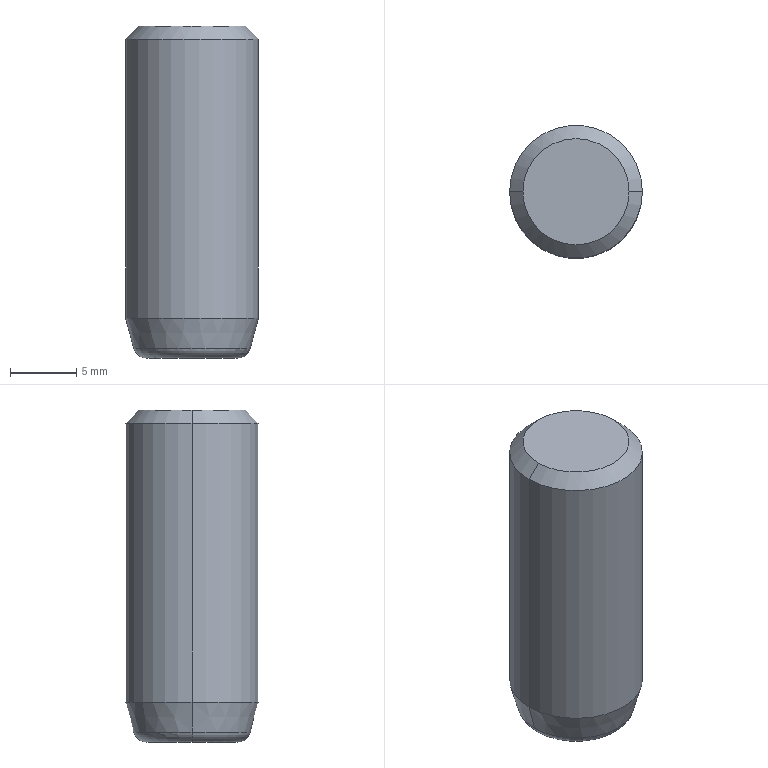Part | NX | features BREP 1 | 1 solid | 10 faces | box 10 x 10 x 25 mm | volume 1910 mm3 | cone 4 | torus 2 | cylinder 2 | plane 2 | commonest cylinder face diameters 10 x2
STEP:
#1=CARTESIAN_POINT('',(-3.429,0.,0.));
#2=VERTEX_POINT('',#1);
#3=CARTESIAN_POINT('',(3.429,0.,0.));
#4=VERTEX_POINT('',#3);
#5=CARTESIAN_POINT('',(0.,0.,0.));
#6=DIRECTION('',(0.,0.,-1.));
#7=DIRECTION('',(1.,0.,0.));
#8=AXIS2_PLACEMENT_3D('',#5,#6,#7);
#9=CIRCLE('',#8,3.429);
#10=EDGE_CURVE('',#2,#4,#9,.T.);
#11=ORIENTED_EDGE('',*,*,#10,.F.);
#12=CARTESIAN_POINT('',(-4.395,0.,0.7412));
#13=VERTEX_POINT('',#12);
#14=CARTESIAN_POINT('',(-3.429,0.,1.));
#15=DIRECTION('',(0.,1.,0.));
#16=DIRECTION('',(-1.,0.,0.));
#17=AXIS2_PLACEMENT_3D('',#14,#15,#16);
#18=CIRCLE('',#17,1.);
#19=EDGE_CURVE('',#13,#2,#18,.F.);
#20=ORIENTED_EDGE('',*,*,#19,.F.);
#21=CARTESIAN_POINT('',(4.395,0.,0.7412));
#22=VERTEX_POINT('',#21);
#23=CARTESIAN_POINT('',(0.,0.,0.7412));
#24=DIRECTION('',(0.,0.,1.));
#25=DIRECTION('',(1.,0.,0.));
#26=AXIS2_PLACEMENT_3D('',#23,#24,#25);
#27=CIRCLE('',#26,4.395);
#28=EDGE_CURVE('',#22,#13,#27,.T.);
#29=ORIENTED_EDGE('',*,*,#28,.F.);
#30=CARTESIAN_POINT('',(3.429,0.,1.));
#31=DIRECTION('',(0.,-1.,0.));
#32=DIRECTION('',(0.,0.,-1.));
#33=AXIS2_PLACEMENT_3D('',#30,#31,#32);
#34=CIRCLE('',#33,1.);
#35=EDGE_CURVE('',#22,#4,#34,.F.);
#36=ORIENTED_EDGE('',*,*,#35,.T.);
#37=EDGE_LOOP('',(#11,#20,#29,#36));
#38=FACE_BOUND('',#37,.T.);
#39=CARTESIAN_POINT('',(0.,0.,1.));
#40=DIRECTION('',(0.,0.,1.));
#41=DIRECTION('',(1.,0.,0.));
#42=AXIS2_PLACEMENT_3D('',#39,#40,#41);
#43=TOROIDAL_SURFACE('',#42,3.429,1.);
#44=ADVANCED_FACE('',(#38),#43,.T.);
#45=ORIENTED_EDGE('',*,*,#28,.T.);
#46=CARTESIAN_POINT('',(-5.,0.,3.));
#47=VERTEX_POINT('',#46);
#48=CARTESIAN_POINT('',(-5.,0.,3.));
#49=DIRECTION('',(-0.2588,0.,0.9659));
#50=VECTOR('',#49,1000.);
#51=LINE('',#48,#50);
#52=EDGE_CURVE('',#47,#13,#51,.F.);
#53=ORIENTED_EDGE('',*,*,#52,.F.);
#54=CARTESIAN_POINT('',(5.,0.,3.));
#55=VERTEX_POINT('',#54);
#56=CARTESIAN_POINT('',(0.,0.,3.));
#57=DIRECTION('',(0.,0.,1.));
#58=DIRECTION('',(1.,0.,0.));
#59=AXIS2_PLACEMENT_3D('',#56,#57,#58);
#60=CIRCLE('',#59,5.);
#61=EDGE_CURVE('',#55,#47,#60,.T.);
#62=ORIENTED_EDGE('',*,*,#61,.F.);
#63=CARTESIAN_POINT('',(5.,0.,3.));
#64=DIRECTION('',(0.2588,0.,0.9659));
#65=VECTOR('',#64,1000.);
#66=LINE('',#63,#65);
#67=EDGE_CURVE('',#55,#22,#66,.F.);
#68=ORIENTED_EDGE('',*,*,#67,.T.);
#69=EDGE_LOOP('',(#45,#53,#62,#68));
#70=FACE_BOUND('',#69,.T.);
#71=CARTESIAN_POINT('',(0.,0.,3.));
#72=DIRECTION('',(0.,0.,1.));
#73=DIRECTION('',(1.,0.,0.));
#74=AXIS2_PLACEMENT_3D('',#71,#72,#73);
#75=CONICAL_SURFACE('',#74,5.,0.2618);
#76=ADVANCED_FACE('',(#70),#75,.T.);
#77=CARTESIAN_POINT('',(4.,0.,25.));
#78=VERTEX_POINT('',#77);
#79=CARTESIAN_POINT('',(-4.,0.,25.));
#80=VERTEX_POINT('',#79);
#81=CARTESIAN_POINT('',(0.,0.,25.));
#82=DIRECTION('',(0.,0.,1.));
#83=DIRECTION('',(1.,0.,0.));
#84=AXIS2_PLACEMENT_3D('',#81,#82,#83);
#85=CIRCLE('',#84,4.);
#86=EDGE_CURVE('',#78,#80,#85,.T.);
#87=ORIENTED_EDGE('',*,*,#86,.F.);
#88=CARTESIAN_POINT('',(5.,0.,24.));
#89=VERTEX_POINT('',#88);
#90=CARTESIAN_POINT('',(4.,0.,25.));
#91=DIRECTION('',(0.7071,0.,-0.7071));
#92=VECTOR('',#91,1000.);
#93=LINE('',#90,#92);
#94=EDGE_CURVE('',#78,#89,#93,.T.);
#95=ORIENTED_EDGE('',*,*,#94,.T.);
#96=CARTESIAN_POINT('',(-5.,0.,24.));
#97=VERTEX_POINT('',#96);
#98=CARTESIAN_POINT('',(0.,0.,24.));
#99=DIRECTION('',(0.,0.,-1.));
#100=DIRECTION('',(1.,0.,0.));
#101=AXIS2_PLACEMENT_3D('',#98,#99,#100);
#102=CIRCLE('',#101,5.);
#103=EDGE_CURVE('',#97,#89,#102,.T.);
#104=ORIENTED_EDGE('',*,*,#103,.F.);
#105=CARTESIAN_POINT('',(-4.,0.,25.));
#106=DIRECTION('',(-0.7071,0.,-0.7071));
#107=VECTOR('',#106,1000.);
#108=LINE('',#105,#107);
#109=EDGE_CURVE('',#80,#97,#108,.T.);
#110=ORIENTED_EDGE('',*,*,#109,.F.);
#111=EDGE_LOOP('',(#87,#95,#104,#110));
#112=FACE_BOUND('',#111,.T.);
#113=CARTESIAN_POINT('',(0.,0.,25.));
#114=DIRECTION('',(0.,0.,-1.));
#115=DIRECTION('',(-1.,0.,0.));
#116=AXIS2_PLACEMENT_3D('',#113,#114,#115);
#117=CONICAL_SURFACE('',#116,4.,0.7854);
#118=ADVANCED_FACE('',(#112),#117,.T.);
#119=ORIENTED_EDGE('',*,*,#103,.T.);
#120=CARTESIAN_POINT('',(5.,0.,25.));
#121=DIRECTION('',(0.,0.,-1.));
#122=VECTOR('',#121,1000.);
#123=LINE('',#120,#122);
#124=EDGE_CURVE('',#89,#55,#123,.T.);
#125=ORIENTED_EDGE('',*,*,#124,.T.);
#126=ORIENTED_EDGE('',*,*,#61,.T.);
#127=CARTESIAN_POINT('',(-5.,0.,25.));
#128=DIRECTION('',(0.,0.,-1.));
#129=VECTOR('',#128,1000.);
#130=LINE('',#127,#129);
#131=EDGE_CURVE('',#97,#47,#130,.T.);
#132=ORIENTED_EDGE('',*,*,#131,.F.);
#133=EDGE_LOOP('',(#119,#125,#126,#132));
#134=FACE_BOUND('',#133,.T.);
#135=CARTESIAN_POINT('',(0.,0.,25.));
#136=DIRECTION('',(0.,0.,-1.));
#137=DIRECTION('',(-1.,0.,0.));
#138=AXIS2_PLACEMENT_3D('',#135,#136,#137);
#139=CYLINDRICAL_SURFACE('',#138,5.);
#140=ADVANCED_FACE('',(#134),#139,.T.);
#141=ORIENTED_EDGE('',*,*,#124,.F.);
#142=CARTESIAN_POINT('',(0.,0.,24.));
#143=DIRECTION('',(0.,0.,-1.));
#144=DIRECTION('',(1.,0.,0.));
#145=AXIS2_PLACEMENT_3D('',#142,#143,#144);
#146=CIRCLE('',#145,5.);
#147=EDGE_CURVE('',#89,#97,#146,.T.);
#148=ORIENTED_EDGE('',*,*,#147,.T.);
#149=ORIENTED_EDGE('',*,*,#131,.T.);
#150=CARTESIAN_POINT('',(0.,0.,3.));
#151=DIRECTION('',(0.,0.,1.));
#152=DIRECTION('',(1.,0.,0.));
#153=AXIS2_PLACEMENT_3D('',#150,#151,#152);
#154=CIRCLE('',#153,5.);
#155=EDGE_CURVE('',#47,#55,#154,.T.);
#156=ORIENTED_EDGE('',*,*,#155,.T.);
#157=EDGE_LOOP('',(#141,#148,#149,#156));
#158=FACE_BOUND('',#157,.T.);
#159=CARTESIAN_POINT('',(0.,0.,25.));
#160=DIRECTION('',(0.,0.,-1.));
#161=DIRECTION('',(-1.,0.,0.));
#162=AXIS2_PLACEMENT_3D('',#159,#160,#161);
#163=CYLINDRICAL_SURFACE('',#162,5.);
#164=ADVANCED_FACE('',(#158),#163,.T.);
#165=CARTESIAN_POINT('',(0.,0.,25.));
#166=DIRECTION('',(0.,0.,1.));
#167=DIRECTION('',(1.,0.,0.));
#168=AXIS2_PLACEMENT_3D('',#165,#166,#167);
#169=CIRCLE('',#168,4.);
#170=EDGE_CURVE('',#80,#78,#169,.T.);
#171=ORIENTED_EDGE('',*,*,#170,.T.);
#172=ORIENTED_EDGE('',*,*,#86,.T.);
#173=EDGE_LOOP('',(#171,#172));
#174=FACE_BOUND('',#173,.T.);
#175=CARTESIAN_POINT('',(0.,0.,25.));
#176=DIRECTION('',(0.,0.,1.));
#177=DIRECTION('',(1.,0.,0.));
#178=AXIS2_PLACEMENT_3D('',#175,#176,#177);
#179=PLANE('',#178);
#180=ADVANCED_FACE('',(#174),#179,.T.);
#181=CARTESIAN_POINT('',(0.,0.,0.));
#182=DIRECTION('',(0.,0.,-1.));
#183=DIRECTION('',(1.,0.,0.));
#184=AXIS2_PLACEMENT_3D('',#181,#182,#183);
#185=CIRCLE('',#184,3.429);
#186=EDGE_CURVE('',#4,#2,#185,.T.);
#187=ORIENTED_EDGE('',*,*,#186,.T.);
#188=ORIENTED_EDGE('',*,*,#10,.T.);
#189=EDGE_LOOP('',(#187,#188));
#190=FACE_BOUND('',#189,.T.);
#191=CARTESIAN_POINT('',(0.,0.,0.));
#192=DIRECTION('',(0.,0.,1.));
#193=DIRECTION('',(1.,0.,0.));
#194=AXIS2_PLACEMENT_3D('',#191,#192,#193);
#195=PLANE('',#194);
#196=ADVANCED_FACE('',(#190),#195,.F.);
#197=ORIENTED_EDGE('',*,*,#94,.F.);
#198=ORIENTED_EDGE('',*,*,#170,.F.);
#199=ORIENTED_EDGE('',*,*,#109,.T.);
#200=ORIENTED_EDGE('',*,*,#147,.F.);
#201=EDGE_LOOP('',(#197,#198,#199,#200));
#202=FACE_BOUND('',#201,.T.);
#203=CARTESIAN_POINT('',(0.,0.,25.));
#204=DIRECTION('',(0.,0.,-1.));
#205=DIRECTION('',(-1.,0.,0.));
#206=AXIS2_PLACEMENT_3D('',#203,#204,#205);
#207=CONICAL_SURFACE('',#206,4.,0.7854);
#208=ADVANCED_FACE('',(#202),#207,.T.);
#209=ORIENTED_EDGE('',*,*,#52,.T.);
#210=CARTESIAN_POINT('',(0.,0.,0.7412));
#211=DIRECTION('',(0.,0.,1.));
#212=DIRECTION('',(1.,0.,0.));
#213=AXIS2_PLACEMENT_3D('',#210,#211,#212);
#214=CIRCLE('',#213,4.395);
#215=EDGE_CURVE('',#13,#22,#214,.T.);
#216=ORIENTED_EDGE('',*,*,#215,.T.);
#217=ORIENTED_EDGE('',*,*,#67,.F.);
#218=ORIENTED_EDGE('',*,*,#155,.F.);
#219=EDGE_LOOP('',(#209,#216,#217,#218));
#220=FACE_BOUND('',#219,.T.);
#221=CARTESIAN_POINT('',(0.,0.,3.));
#222=DIRECTION('',(0.,0.,1.));
#223=DIRECTION('',(1.,0.,0.));
#224=AXIS2_PLACEMENT_3D('',#221,#222,#223);
#225=CONICAL_SURFACE('',#224,5.,0.2618);
#226=ADVANCED_FACE('',(#220),#225,.T.);
#227=ORIENTED_EDGE('',*,*,#19,.T.);
#228=ORIENTED_EDGE('',*,*,#186,.F.);
#229=ORIENTED_EDGE('',*,*,#35,.F.);
#230=ORIENTED_EDGE('',*,*,#215,.F.);
#231=EDGE_LOOP('',(#227,#228,#229,#230));
#232=FACE_BOUND('',#231,.T.);
#233=CARTESIAN_POINT('',(0.,0.,1.));
#234=DIRECTION('',(0.,0.,1.));
#235=DIRECTION('',(1.,0.,0.));
#236=AXIS2_PLACEMENT_3D('',#233,#234,#235);
#237=TOROIDAL_SURFACE('',#236,3.429,1.);
#238=ADVANCED_FACE('',(#232),#237,.T.);
#239=CLOSED_SHELL('',(#44,#76,#118,#140,#164,#180,#196,#208,#226,#238));
#240=MANIFOLD_SOLID_BREP('',#239);
#241=(LENGTH_UNIT()NAMED_UNIT(*)SI_UNIT(.MILLI.,.METRE.));
#242=UNCERTAINTY_MEASURE_WITH_UNIT(LENGTH_MEASURE(0.00001),#241,'','');
#243=(NAMED_UNIT(*)PLANE_ANGLE_UNIT()SI_UNIT($,.RADIAN.));
#244=(NAMED_UNIT(*)SI_UNIT($,.STERADIAN.)SOLID_ANGLE_UNIT());
#245=(GEOMETRIC_REPRESENTATION_CONTEXT(3)GLOBAL_UNCERTAINTY_ASSIGNED_CONTEXT((#242))GLOBAL_UNIT_ASSIGNED_CONTEXT((#241,#243,#244))REPRESENTATION_CONTEXT('',''));
#246=ADVANCED_BREP_SHAPE_REPRESENTATION('',(#240),#245);